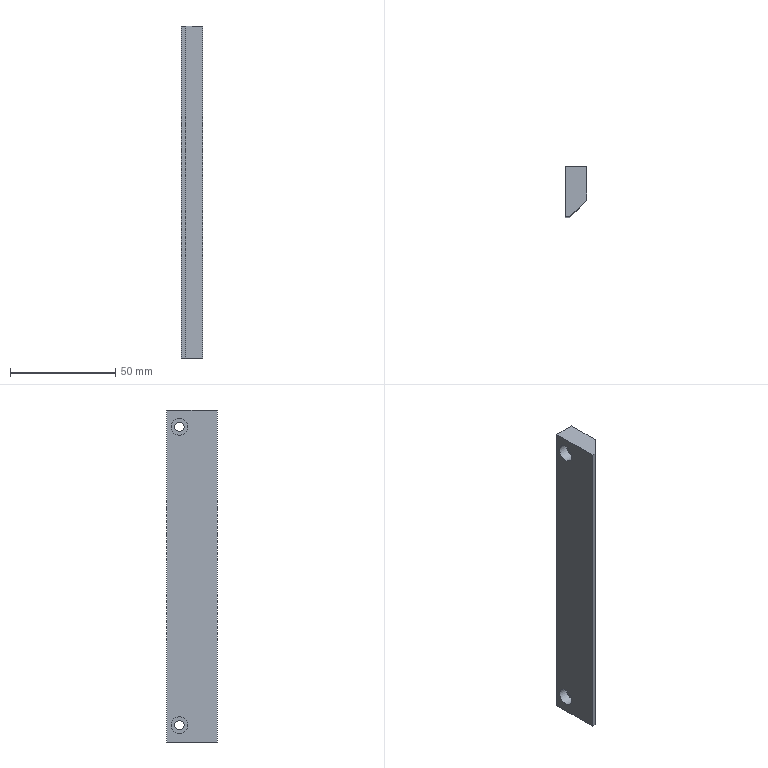Part | NX | 1 solid | 13 faces | box 10 x 24 x 158 mm | volume 32230 mm3 | plane 9 | cylinder 4 | commonest cylinder face diameters 4.5 x2 8 x2
STEP:
#1=CARTESIAN_POINT('',(5.,18.,73.25));
#2=VERTEX_POINT('',#1);
#3=CARTESIAN_POINT('',(5.,18.,71.));
#4=DIRECTION('',(-1.,0.,0.));
#5=DIRECTION('',(0.,0.,1.));
#6=AXIS2_PLACEMENT_3D('',#3,#4,#5);
#7=CIRCLE('',#6,2.25);
#8=EDGE_CURVE('',#2,#2,#7,.T.);
#9=ORIENTED_EDGE('',*,*,#8,.T.);
#10=EDGE_LOOP('',(#9));
#11=FACE_BOUND('',#10,.T.);
#12=CARTESIAN_POINT('',(5.,18.,-68.75));
#13=VERTEX_POINT('',#12);
#14=CARTESIAN_POINT('',(5.,18.,-71.));
#15=DIRECTION('',(-1.,0.,0.));
#16=DIRECTION('',(0.,0.,1.));
#17=AXIS2_PLACEMENT_3D('',#14,#15,#16);
#18=CIRCLE('',#17,2.25);
#19=EDGE_CURVE('',#13,#13,#18,.T.);
#20=ORIENTED_EDGE('',*,*,#19,.T.);
#21=EDGE_LOOP('',(#20));
#22=FACE_BOUND('',#21,.T.);
#23=CARTESIAN_POINT('',(5.,8.,79.));
#24=VERTEX_POINT('',#23);
#25=CARTESIAN_POINT('',(5.,8.,-79.));
#26=VERTEX_POINT('',#25);
#27=CARTESIAN_POINT('',(5.,8.,-174.));
#28=DIRECTION('',(0.,0.,-1.));
#29=VECTOR('',#28,1000.);
#30=LINE('',#27,#29);
#31=EDGE_CURVE('',#24,#26,#30,.T.);
#32=ORIENTED_EDGE('',*,*,#31,.T.);
#33=CARTESIAN_POINT('',(5.,24.,-79.));
#34=VERTEX_POINT('',#33);
#35=CARTESIAN_POINT('',(5.,24.,-79.));
#36=DIRECTION('',(0.,1.,0.));
#37=VECTOR('',#36,1000.);
#38=LINE('',#35,#37);
#39=EDGE_CURVE('',#26,#34,#38,.T.);
#40=ORIENTED_EDGE('',*,*,#39,.T.);
#41=CARTESIAN_POINT('',(5.,24.,79.));
#42=VERTEX_POINT('',#41);
#43=CARTESIAN_POINT('',(5.,24.,174.));
#44=DIRECTION('',(0.,0.,-1.));
#45=VECTOR('',#44,1000.);
#46=LINE('',#43,#45);
#47=EDGE_CURVE('',#42,#34,#46,.T.);
#48=ORIENTED_EDGE('',*,*,#47,.F.);
#49=CARTESIAN_POINT('',(5.,24.,79.));
#50=DIRECTION('',(0.,-1.,0.));
#51=VECTOR('',#50,1000.);
#52=LINE('',#49,#51);
#53=EDGE_CURVE('',#42,#24,#52,.T.);
#54=ORIENTED_EDGE('',*,*,#53,.T.);
#55=EDGE_LOOP('',(#32,#40,#48,#54));
#56=FACE_BOUND('',#55,.T.);
#57=CARTESIAN_POINT('',(5.,24.,174.));
#58=DIRECTION('',(-1.,0.,0.));
#59=DIRECTION('',(0.,0.,1.));
#60=AXIS2_PLACEMENT_3D('',#57,#58,#59);
#61=PLANE('',#60);
#62=ADVANCED_FACE('',(#11,#22,#56),#61,.F.);
#63=CARTESIAN_POINT('',(-5.,18.,75.));
#64=VERTEX_POINT('',#63);
#65=CARTESIAN_POINT('',(-5.,18.,71.));
#66=DIRECTION('',(-1.,0.,0.));
#67=DIRECTION('',(0.,0.,1.));
#68=AXIS2_PLACEMENT_3D('',#65,#66,#67);
#69=CIRCLE('',#68,4.);
#70=EDGE_CURVE('',#64,#64,#69,.T.);
#71=ORIENTED_EDGE('',*,*,#70,.F.);
#72=EDGE_LOOP('',(#71));
#73=FACE_BOUND('',#72,.T.);
#74=CARTESIAN_POINT('',(-5.,18.,-67.));
#75=VERTEX_POINT('',#74);
#76=CARTESIAN_POINT('',(-5.,18.,-71.));
#77=DIRECTION('',(-1.,0.,0.));
#78=DIRECTION('',(0.,0.,1.));
#79=AXIS2_PLACEMENT_3D('',#76,#77,#78);
#80=CIRCLE('',#79,4.);
#81=EDGE_CURVE('',#75,#75,#80,.T.);
#82=ORIENTED_EDGE('',*,*,#81,.F.);
#83=EDGE_LOOP('',(#82));
#84=FACE_BOUND('',#83,.T.);
#85=CARTESIAN_POINT('',(-5.,24.,-79.));
#86=VERTEX_POINT('',#85);
#87=CARTESIAN_POINT('',(-5.,24.,79.));
#88=VERTEX_POINT('',#87);
#89=CARTESIAN_POINT('',(-5.,24.,174.));
#90=DIRECTION('',(0.,0.,1.));
#91=VECTOR('',#90,1000.);
#92=LINE('',#89,#91);
#93=EDGE_CURVE('',#86,#88,#92,.T.);
#94=ORIENTED_EDGE('',*,*,#93,.F.);
#95=CARTESIAN_POINT('',(-5.,0.,-79.));
#96=VERTEX_POINT('',#95);
#97=CARTESIAN_POINT('',(-5.,24.,-79.));
#98=DIRECTION('',(0.,1.,0.));
#99=VECTOR('',#98,1000.);
#100=LINE('',#97,#99);
#101=EDGE_CURVE('',#96,#86,#100,.T.);
#102=ORIENTED_EDGE('',*,*,#101,.F.);
#103=CARTESIAN_POINT('',(-5.,0.,79.));
#104=VERTEX_POINT('',#103);
#105=CARTESIAN_POINT('',(-5.,0.,174.));
#106=DIRECTION('',(0.,0.,1.));
#107=VECTOR('',#106,1000.);
#108=LINE('',#105,#107);
#109=EDGE_CURVE('',#96,#104,#108,.T.);
#110=ORIENTED_EDGE('',*,*,#109,.T.);
#111=CARTESIAN_POINT('',(-5.,24.,79.));
#112=DIRECTION('',(0.,-1.,0.));
#113=VECTOR('',#112,1000.);
#114=LINE('',#111,#113);
#115=EDGE_CURVE('',#88,#104,#114,.T.);
#116=ORIENTED_EDGE('',*,*,#115,.F.);
#117=EDGE_LOOP('',(#94,#102,#110,#116));
#118=FACE_BOUND('',#117,.T.);
#119=CARTESIAN_POINT('',(-5.,24.,174.));
#120=DIRECTION('',(1.,0.,0.));
#121=DIRECTION('',(0.,0.,-1.));
#122=AXIS2_PLACEMENT_3D('',#119,#120,#121);
#123=PLANE('',#122);
#124=ADVANCED_FACE('',(#73,#84,#118),#123,.F.);
#125=ORIENTED_EDGE('',*,*,#47,.T.);
#126=CARTESIAN_POINT('',(5.,24.,-79.));
#127=DIRECTION('',(-1.,0.,0.));
#128=VECTOR('',#127,1000.);
#129=LINE('',#126,#128);
#130=EDGE_CURVE('',#34,#86,#129,.T.);
#131=ORIENTED_EDGE('',*,*,#130,.T.);
#132=ORIENTED_EDGE('',*,*,#93,.T.);
#133=CARTESIAN_POINT('',(5.,24.,79.));
#134=DIRECTION('',(-1.,0.,0.));
#135=VECTOR('',#134,1000.);
#136=LINE('',#133,#135);
#137=EDGE_CURVE('',#42,#88,#136,.T.);
#138=ORIENTED_EDGE('',*,*,#137,.F.);
#139=EDGE_LOOP('',(#125,#131,#132,#138));
#140=FACE_BOUND('',#139,.T.);
#141=CARTESIAN_POINT('',(0.,24.,0.));
#142=DIRECTION('',(0.,-1.,0.));
#143=DIRECTION('',(0.,0.,-1.));
#144=AXIS2_PLACEMENT_3D('',#141,#142,#143);
#145=PLANE('',#144);
#146=ADVANCED_FACE('',(#140),#145,.F.);
#147=CARTESIAN_POINT('',(-3.,0.,-79.));
#148=VERTEX_POINT('',#147);
#149=CARTESIAN_POINT('',(5.,8.,-79.));
#150=DIRECTION('',(-0.7071,-0.7071,0.));
#151=VECTOR('',#150,1000.);
#152=LINE('',#149,#151);
#153=EDGE_CURVE('',#26,#148,#152,.T.);
#154=ORIENTED_EDGE('',*,*,#153,.F.);
#155=ORIENTED_EDGE('',*,*,#31,.F.);
#156=CARTESIAN_POINT('',(-3.,0.,79.));
#157=VERTEX_POINT('',#156);
#158=CARTESIAN_POINT('',(5.,8.,79.));
#159=DIRECTION('',(0.7071,0.7071,0.));
#160=VECTOR('',#159,1000.);
#161=LINE('',#158,#160);
#162=EDGE_CURVE('',#157,#24,#161,.T.);
#163=ORIENTED_EDGE('',*,*,#162,.F.);
#164=CARTESIAN_POINT('',(-3.,0.,174.));
#165=DIRECTION('',(0.,0.,1.));
#166=VECTOR('',#165,1000.);
#167=LINE('',#164,#166);
#168=EDGE_CURVE('',#148,#157,#167,.T.);
#169=ORIENTED_EDGE('',*,*,#168,.F.);
#170=EDGE_LOOP('',(#154,#155,#163,#169));
#171=FACE_BOUND('',#170,.T.);
#172=CARTESIAN_POINT('',(5.,8.,174.));
#173=DIRECTION('',(0.7071,-0.7071,0.));
#174=DIRECTION('',(0.,0.,1.));
#175=AXIS2_PLACEMENT_3D('',#172,#173,#174);
#176=PLANE('',#175);
#177=ADVANCED_FACE('',(#171),#176,.T.);
#178=CARTESIAN_POINT('',(5.,0.,-79.));
#179=DIRECTION('',(-1.,0.,0.));
#180=VECTOR('',#179,1000.);
#181=LINE('',#178,#180);
#182=EDGE_CURVE('',#148,#96,#181,.T.);
#183=ORIENTED_EDGE('',*,*,#182,.F.);
#184=ORIENTED_EDGE('',*,*,#168,.T.);
#185=CARTESIAN_POINT('',(5.,0.,79.));
#186=DIRECTION('',(-1.,0.,0.));
#187=VECTOR('',#186,1000.);
#188=LINE('',#185,#187);
#189=EDGE_CURVE('',#157,#104,#188,.T.);
#190=ORIENTED_EDGE('',*,*,#189,.T.);
#191=ORIENTED_EDGE('',*,*,#109,.F.);
#192=EDGE_LOOP('',(#183,#184,#190,#191));
#193=FACE_BOUND('',#192,.T.);
#194=CARTESIAN_POINT('',(0.,0.,0.));
#195=DIRECTION('',(0.,-1.,0.));
#196=DIRECTION('',(0.,0.,-1.));
#197=AXIS2_PLACEMENT_3D('',#194,#195,#196);
#198=PLANE('',#197);
#199=ADVANCED_FACE('',(#193),#198,.T.);
#200=ORIENTED_EDGE('',*,*,#162,.T.);
#201=ORIENTED_EDGE('',*,*,#53,.F.);
#202=ORIENTED_EDGE('',*,*,#137,.T.);
#203=ORIENTED_EDGE('',*,*,#115,.T.);
#204=ORIENTED_EDGE('',*,*,#189,.F.);
#205=EDGE_LOOP('',(#200,#201,#202,#203,#204));
#206=FACE_BOUND('',#205,.T.);
#207=CARTESIAN_POINT('',(5.,24.,79.));
#208=DIRECTION('',(0.,0.,-1.));
#209=DIRECTION('',(0.,1.,0.));
#210=AXIS2_PLACEMENT_3D('',#207,#208,#209);
#211=PLANE('',#210);
#212=ADVANCED_FACE('',(#206),#211,.F.);
#213=ORIENTED_EDGE('',*,*,#153,.T.);
#214=ORIENTED_EDGE('',*,*,#182,.T.);
#215=ORIENTED_EDGE('',*,*,#101,.T.);
#216=ORIENTED_EDGE('',*,*,#130,.F.);
#217=ORIENTED_EDGE('',*,*,#39,.F.);
#218=EDGE_LOOP('',(#213,#214,#215,#216,#217));
#219=FACE_BOUND('',#218,.T.);
#220=CARTESIAN_POINT('',(5.,24.,-79.));
#221=DIRECTION('',(0.,0.,1.));
#222=DIRECTION('',(0.,-1.,0.));
#223=AXIS2_PLACEMENT_3D('',#220,#221,#222);
#224=PLANE('',#223);
#225=ADVANCED_FACE('',(#219),#224,.F.);
#226=ORIENTED_EDGE('',*,*,#19,.F.);
#227=EDGE_LOOP('',(#226));
#228=FACE_BOUND('',#227,.T.);
#229=CARTESIAN_POINT('',(-0.4,18.,-68.75));
#230=VERTEX_POINT('',#229);
#231=CARTESIAN_POINT('',(-0.4,18.,-71.));
#232=DIRECTION('',(-1.,0.,0.));
#233=DIRECTION('',(0.,0.,1.));
#234=AXIS2_PLACEMENT_3D('',#231,#232,#233);
#235=CIRCLE('',#234,2.25);
#236=EDGE_CURVE('',#230,#230,#235,.T.);
#237=ORIENTED_EDGE('',*,*,#236,.T.);
#238=EDGE_LOOP('',(#237));
#239=FACE_BOUND('',#238,.T.);
#240=CARTESIAN_POINT('',(-5.,18.,-71.));
#241=DIRECTION('',(-1.,0.,0.));
#242=DIRECTION('',(0.,0.,1.));
#243=AXIS2_PLACEMENT_3D('',#240,#241,#242);
#244=CYLINDRICAL_SURFACE('',#243,2.25);
#245=ADVANCED_FACE('',(#228,#239),#244,.F.);
#246=ORIENTED_EDGE('',*,*,#236,.F.);
#247=EDGE_LOOP('',(#246));
#248=FACE_BOUND('',#247,.T.);
#249=CARTESIAN_POINT('',(-0.4,18.,-67.));
#250=VERTEX_POINT('',#249);
#251=CARTESIAN_POINT('',(-0.4,18.,-71.));
#252=DIRECTION('',(-1.,0.,0.));
#253=DIRECTION('',(0.,0.,1.));
#254=AXIS2_PLACEMENT_3D('',#251,#252,#253);
#255=CIRCLE('',#254,4.);
#256=EDGE_CURVE('',#250,#250,#255,.T.);
#257=ORIENTED_EDGE('',*,*,#256,.T.);
#258=EDGE_LOOP('',(#257));
#259=FACE_BOUND('',#258,.T.);
#260=CARTESIAN_POINT('',(-0.4,20.25,-71.));
#261=DIRECTION('',(1.,0.,0.));
#262=DIRECTION('',(0.,0.,-1.));
#263=AXIS2_PLACEMENT_3D('',#260,#261,#262);
#264=PLANE('',#263);
#265=ADVANCED_FACE('',(#248,#259),#264,.F.);
#266=ORIENTED_EDGE('',*,*,#256,.F.);
#267=EDGE_LOOP('',(#266));
#268=FACE_BOUND('',#267,.T.);
#269=ORIENTED_EDGE('',*,*,#81,.T.);
#270=EDGE_LOOP('',(#269));
#271=FACE_BOUND('',#270,.T.);
#272=CARTESIAN_POINT('',(-5.,18.,-71.));
#273=DIRECTION('',(-1.,0.,0.));
#274=DIRECTION('',(0.,0.,1.));
#275=AXIS2_PLACEMENT_3D('',#272,#273,#274);
#276=CYLINDRICAL_SURFACE('',#275,4.);
#277=ADVANCED_FACE('',(#268,#271),#276,.F.);
#278=ORIENTED_EDGE('',*,*,#8,.F.);
#279=EDGE_LOOP('',(#278));
#280=FACE_BOUND('',#279,.T.);
#281=CARTESIAN_POINT('',(-0.4,18.,73.25));
#282=VERTEX_POINT('',#281);
#283=CARTESIAN_POINT('',(-0.4,18.,71.));
#284=DIRECTION('',(-1.,0.,0.));
#285=DIRECTION('',(0.,0.,1.));
#286=AXIS2_PLACEMENT_3D('',#283,#284,#285);
#287=CIRCLE('',#286,2.25);
#288=EDGE_CURVE('',#282,#282,#287,.T.);
#289=ORIENTED_EDGE('',*,*,#288,.T.);
#290=EDGE_LOOP('',(#289));
#291=FACE_BOUND('',#290,.T.);
#292=CARTESIAN_POINT('',(-5.,18.,71.));
#293=DIRECTION('',(-1.,0.,0.));
#294=DIRECTION('',(0.,0.,1.));
#295=AXIS2_PLACEMENT_3D('',#292,#293,#294);
#296=CYLINDRICAL_SURFACE('',#295,2.25);
#297=ADVANCED_FACE('',(#280,#291),#296,.F.);
#298=ORIENTED_EDGE('',*,*,#288,.F.);
#299=EDGE_LOOP('',(#298));
#300=FACE_BOUND('',#299,.T.);
#301=CARTESIAN_POINT('',(-0.4,18.,75.));
#302=VERTEX_POINT('',#301);
#303=CARTESIAN_POINT('',(-0.4,18.,71.));
#304=DIRECTION('',(-1.,0.,0.));
#305=DIRECTION('',(0.,0.,1.));
#306=AXIS2_PLACEMENT_3D('',#303,#304,#305);
#307=CIRCLE('',#306,4.);
#308=EDGE_CURVE('',#302,#302,#307,.T.);
#309=ORIENTED_EDGE('',*,*,#308,.T.);
#310=EDGE_LOOP('',(#309));
#311=FACE_BOUND('',#310,.T.);
#312=CARTESIAN_POINT('',(-0.4,20.25,71.));
#313=DIRECTION('',(1.,0.,0.));
#314=DIRECTION('',(0.,0.,-1.));
#315=AXIS2_PLACEMENT_3D('',#312,#313,#314);
#316=PLANE('',#315);
#317=ADVANCED_FACE('',(#300,#311),#316,.F.);
#318=ORIENTED_EDGE('',*,*,#308,.F.);
#319=EDGE_LOOP('',(#318));
#320=FACE_BOUND('',#319,.T.);
#321=ORIENTED_EDGE('',*,*,#70,.T.);
#322=EDGE_LOOP('',(#321));
#323=FACE_BOUND('',#322,.T.);
#324=CARTESIAN_POINT('',(-5.,18.,71.));
#325=DIRECTION('',(-1.,0.,0.));
#326=DIRECTION('',(0.,0.,1.));
#327=AXIS2_PLACEMENT_3D('',#324,#325,#326);
#328=CYLINDRICAL_SURFACE('',#327,4.);
#329=ADVANCED_FACE('',(#320,#323),#328,.F.);
#330=CLOSED_SHELL('',(#62,#124,#146,#177,#199,#212,#225,#245,#265,#277,#297,#317,#329));
#331=MANIFOLD_SOLID_BREP('',#330);
#332=(LENGTH_UNIT()NAMED_UNIT(*)SI_UNIT(.MILLI.,.METRE.));
#333=UNCERTAINTY_MEASURE_WITH_UNIT(LENGTH_MEASURE(0.00001),#332,'','');
#334=(NAMED_UNIT(*)PLANE_ANGLE_UNIT()SI_UNIT($,.RADIAN.));
#335=(NAMED_UNIT(*)SI_UNIT($,.STERADIAN.)SOLID_ANGLE_UNIT());
#336=(GEOMETRIC_REPRESENTATION_CONTEXT(3)GLOBAL_UNCERTAINTY_ASSIGNED_CONTEXT((#333))GLOBAL_UNIT_ASSIGNED_CONTEXT((#332,#334,#335))REPRESENTATION_CONTEXT('',''));
#337=ADVANCED_BREP_SHAPE_REPRESENTATION('',(#331),#336);